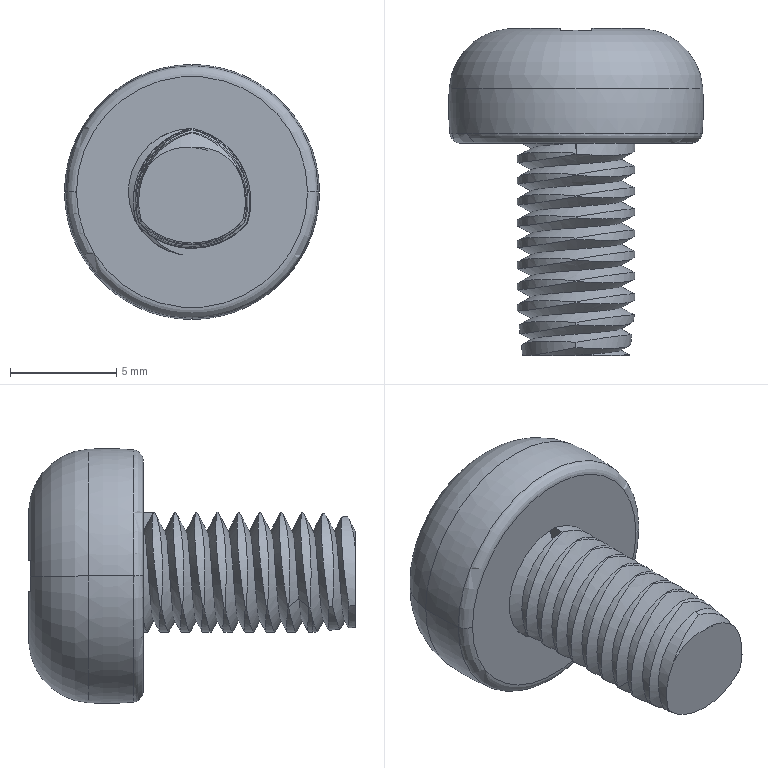Part | NX | features solid 2 | 1 solid | 67 faces | box 12 x 15.4 x 12 mm | volume 693.964 mm3 | cylinder 26 | plane 20 | cone 8 | spline 7 | torus 6 | commonest cylinder face diameters 7 x25 6 x1